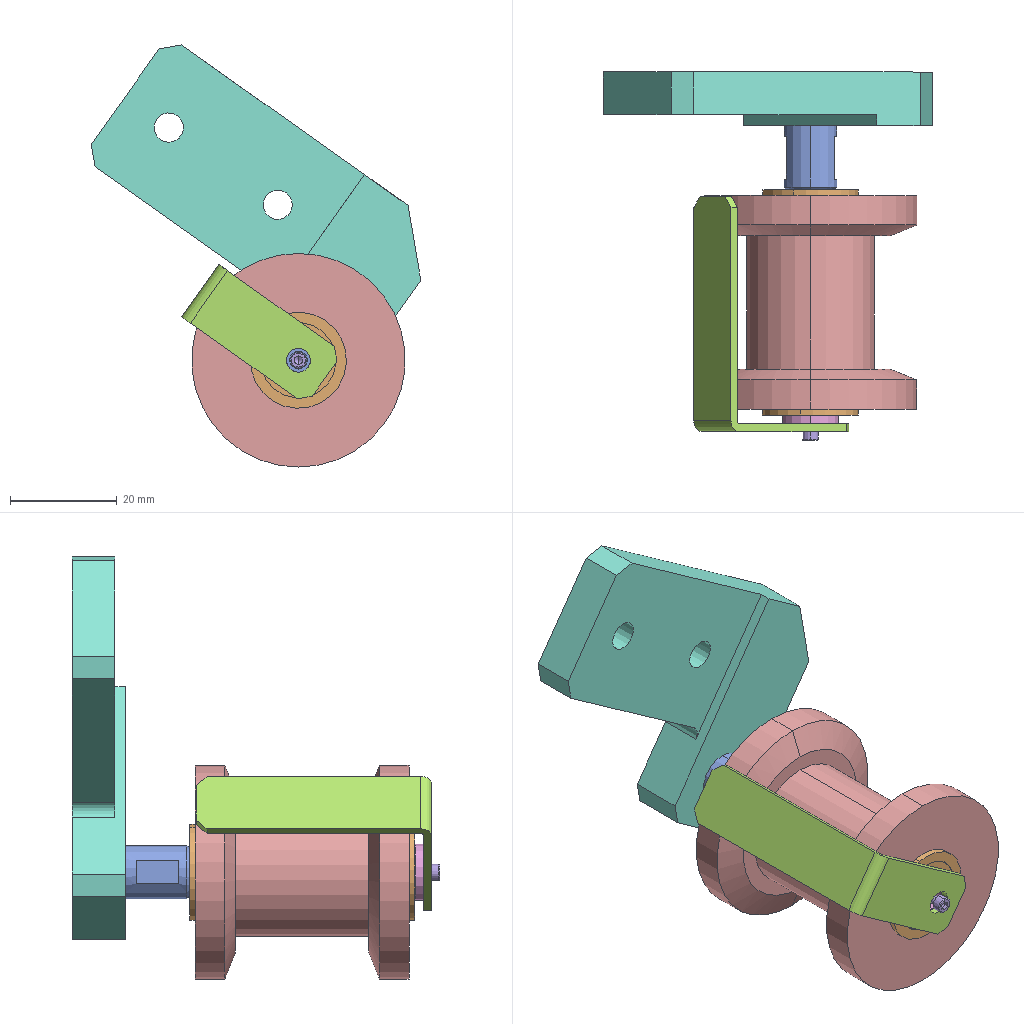Assembly | SolidWorks | 7 different items | 8 placed | box 62 x 69 x 79 mm
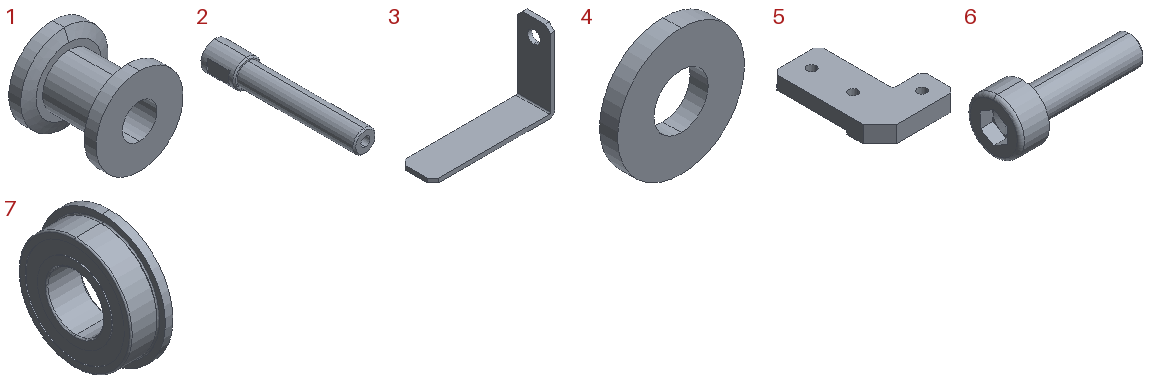Parts list (item | quantity | size | volume | features):
1 | x1 | 40 x 40 x 40 mm | 20965 mm3 | features Chamfer 1, Extrusion 1, RevCut 1
2 | x1 | 10 x 54.3 x 10 mm | 2772 mm3 | features 3DProfileFeature 2, HoleWzd 2, ICE 2, Chamfer 1, Extrusion 1
3 | x1 | 44 x 12 x 28.5 mm | 1232 mm3 | features Fillet 2, Chamfer 1, Extrusion 1, ICE 1
4 | x1 | 10.5 x 1.5 x 10.5 mm | 106.029 mm3 | features Extrusion 1
5 | x1 | 46 x 65 x 10 mm | 18007 mm3 | features ICE 4, Chamfer 2, Extrusion 1, Fillet 1
6 | x1 | 7.6 x 3 x 3 mm | 21.652 mm3 | features Fillet 2, RevCut 2, Boss 1, Chamfer 1, Cut 1, Extrusion 1, LPattern 1
7 | x2 | 5 x 18 x 18 mm | 785.119 mm3 | features RefAxis 3, 3DProfileFeature 1, Revolution 1
Mates (type | each side: item.copy, entity, surface, feature):
Concentric | 1.1 face cylinder Boss-Extrude1 | 7.1 face cylinder Revolve1
Coincident | 1.1 face plane Boss-Extrude1 | 7.2 face plane Revolve1
Concentric | 1.1 face cylinder Boss-Extrude1 | 7.2 face cylinder Revolve1
Coincident | 7.2 face plane Revolve1 | 2.1 face plane Boss-Extrude2
Concentric | 7.2 face cylinder Revolve1 | 2.1 face cylinder Boss-Extrude1
Coincident | 1.1 face plane Boss-Extrude1 | 7.1 face plane Revolve1
Concentric | 2.1 face cylinder M4 Tapped Hole1 | 3.1 face cylinder Cut-Extrude1
DistanceDim | 2.1 face plane Boss-Extrude1 | 3.1 face plane Boss-Extrude1
Concentric | 3.1 face cylinder Cut-Extrude1 | 6.1 face cylinder BaseBody
Coincident | 3.1 face plane Boss-Extrude1 | 6.1 face plane BaseHead
Coincident | 2.1 face plane Boss-Extrude1 | 4.1 face plane Boss-Extrude1
Concentric | 6.1 face cylinder BaseBody | 4.1 face cylinder Boss-Extrude1
Concentric | 2.1 face cylinder M5 Tapped Hole1 | 5.1 face cylinder Cut-Extrude1
Parallel | 3.1 face plane Boss-Extrude1 | 5.1 face plane Boss-Extrude1
Coincident | 2.1 face plane Boss-Extrude2 | 5.1 face plane Boss-Extrude2